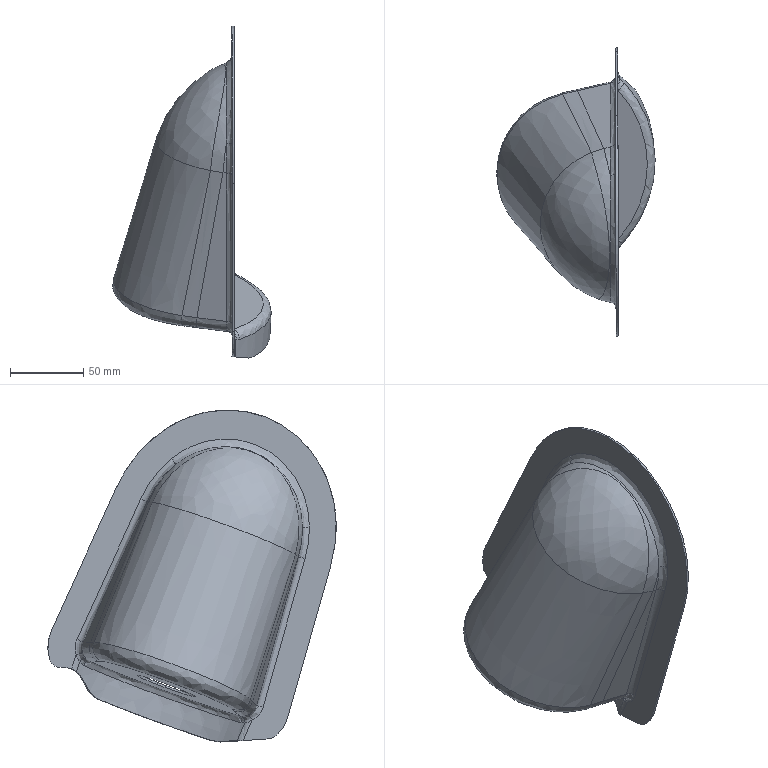Part | 1 solid | 92 faces | box 107.959 x 196.302 x 226.093 mm | volume 76079 mm3 | spline 78 | plane 6 | other 6 | cylinder 2 | commonest cylinder face diameters 37 x2